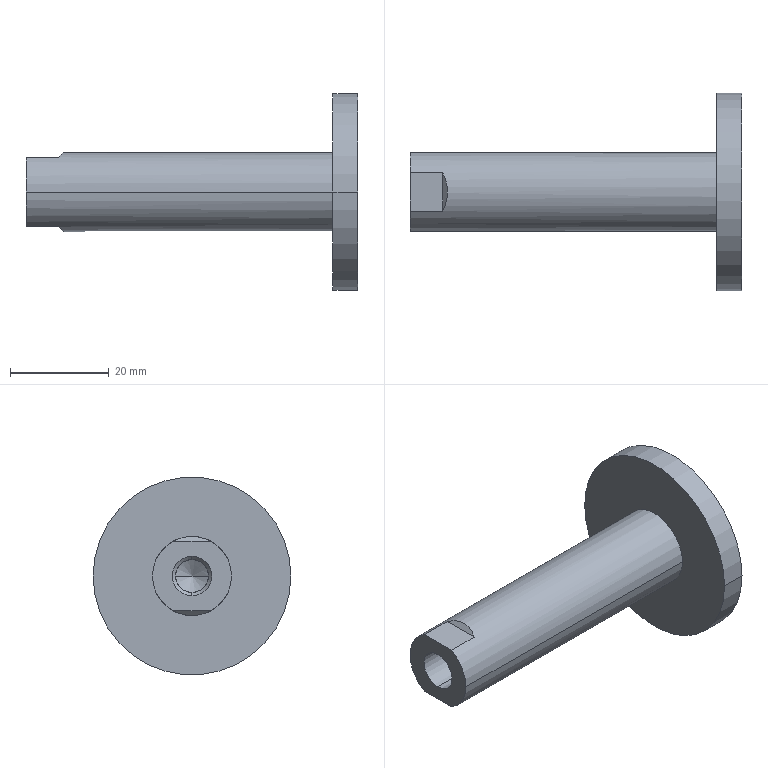Part | STEP file | [25A-CDQ2B40-45C-CYROD] | 1 solid | 19 faces | box 67 x 40 x 40 mm | volume 18078 mm3 | cylinder 8 | plane 7 | cone 4 | commonest cylinder face diameters 6.647 x2 8 x2 16 x2 40 x2
STEP:
#1=CARTESIAN_POINT('',(0.,0.,0.));
#2=DIRECTION('',(0.,0.,1.));
#3=DIRECTION('',(1.,0.,0.));
#4=AXIS2_PLACEMENT_3D('',#1,#2,#3);
#5=CARTESIAN_POINT('',(1.41,0.,-3.323));
#6=VERTEX_POINT('',#5);
#7=CARTESIAN_POINT('',(1.41,3.324,0.));
#8=VERTEX_POINT('',#7);
#9=CARTESIAN_POINT('',(1.41,0.,0.));
#10=DIRECTION('',(1.,0.,0.));
#11=DIRECTION('',(0.,0.,-1.));
#12=AXIS2_PLACEMENT_3D('',#9,#10,#11);
#13=CIRCLE('',#12,3.324);
#14=CARTESIAN_POINT('',(-0.1618,0.,0.));
#15=DIRECTION('',(1.,0.,0.));
#16=DIRECTION('',(0.,1.,0.));
#17=AXIS2_PLACEMENT_3D('',#14,#15,#16);
#18=CYLINDRICAL_SURFACE('',#17,3.324);
#19=CARTESIAN_POINT('',(4.712,1.571));
#20=DIRECTION('',(1.,0.));
#21=VECTOR('',#20,1.);
#22=LINE('',#19,#21);
#23=(GEOMETRIC_REPRESENTATION_CONTEXT(2)PARAMETRIC_REPRESENTATION_CONTEXT()REPRESENTATION_CONTEXT('',''));
#24=DEFINITIONAL_REPRESENTATION('',(#22),#23);
#25=PCURVE('',#18,#24);
#26=CARTESIAN_POINT('',(0.733,0.,0.));
#27=DIRECTION('',(-1.,0.,0.));
#28=DIRECTION('',(0.,0.,-1.));
#29=AXIS2_PLACEMENT_3D('',#26,#27,#28);
#30=CONICAL_SURFACE('',#29,4.,0.7854);
#31=CARTESIAN_POINT('',(6.283,-0.6765));
#32=DIRECTION('',(-1.,0.));
#33=VECTOR('',#32,1.);
#34=LINE('',#31,#33);
#35=(GEOMETRIC_REPRESENTATION_CONTEXT(2)PARAMETRIC_REPRESENTATION_CONTEXT()REPRESENTATION_CONTEXT('',''));
#36=DEFINITIONAL_REPRESENTATION('',(#34),#35);
#37=PCURVE('',#30,#36);
#38=SURFACE_CURVE('',#13,(#25,#37),.PCURVE_S1.);
#39=EDGE_CURVE('',#6,#8,#38,.T.);
#40=ORIENTED_EDGE('',*,*,#39,.T.);
#41=CARTESIAN_POINT('',(6.,3.324,0.));
#42=VERTEX_POINT('',#41);
#43=CARTESIAN_POINT('',(-0.1618,3.324,0.));
#44=DIRECTION('',(1.,0.,0.));
#45=VECTOR('',#44,1.);
#46=LINE('',#43,#45);
#47=CARTESIAN_POINT('',(6.283,0.));
#48=DIRECTION('',(0.,1.));
#49=VECTOR('',#48,1.);
#50=LINE('',#47,#49);
#51=(GEOMETRIC_REPRESENTATION_CONTEXT(2)PARAMETRIC_REPRESENTATION_CONTEXT()REPRESENTATION_CONTEXT('',''));
#52=DEFINITIONAL_REPRESENTATION('',(#50),#51);
#53=PCURVE('',#18,#52);
#54=CARTESIAN_POINT('',(-0.1618,0.,0.));
#55=DIRECTION('',(1.,0.,0.));
#56=DIRECTION('',(0.,1.,0.));
#57=AXIS2_PLACEMENT_3D('',#54,#55,#56);
#58=CYLINDRICAL_SURFACE('',#57,3.324);
#59=CARTESIAN_POINT('',(0.,0.));
#60=DIRECTION('',(0.,1.));
#61=VECTOR('',#60,1.);
#62=LINE('',#59,#61);
#63=(GEOMETRIC_REPRESENTATION_CONTEXT(2)PARAMETRIC_REPRESENTATION_CONTEXT()REPRESENTATION_CONTEXT('',''));
#64=DEFINITIONAL_REPRESENTATION('',(#62),#63);
#65=PCURVE('',#58,#64);
#66=SURFACE_CURVE('',#46,(#53,#65),.PCURVE_S1.);
#67=EDGE_CURVE('',#8,#42,#66,.T.);
#68=ORIENTED_EDGE('',*,*,#67,.T.);
#69=CARTESIAN_POINT('',(6.,-3.324,0.));
#70=VERTEX_POINT('',#69);
#71=CARTESIAN_POINT('',(6.,0.,0.));
#72=DIRECTION('',(-1.,0.,0.));
#73=DIRECTION('',(0.,1.,0.));
#74=AXIS2_PLACEMENT_3D('',#71,#72,#73);
#75=CIRCLE('',#74,3.324);
#76=CARTESIAN_POINT('',(6.283,6.162));
#77=DIRECTION('',(-1.,0.));
#78=VECTOR('',#77,1.);
#79=LINE('',#76,#78);
#80=(GEOMETRIC_REPRESENTATION_CONTEXT(2)PARAMETRIC_REPRESENTATION_CONTEXT()REPRESENTATION_CONTEXT('',''));
#81=DEFINITIONAL_REPRESENTATION('',(#79),#80);
#82=PCURVE('',#18,#81);
#83=CARTESIAN_POINT('',(-992.081,0.,0.));
#84=DIRECTION('',(-1.,0.,0.));
#85=DIRECTION('',(0.,-1.,0.));
#86=AXIS2_PLACEMENT_3D('',#83,#84,#85);
#87=CONICAL_SURFACE('',#86,1732.051,1.047);
#88=CARTESIAN_POINT('',(3.142,-998.081));
#89=DIRECTION('',(1.,0.));
#90=VECTOR('',#89,1.);
#91=LINE('',#88,#90);
#92=(GEOMETRIC_REPRESENTATION_CONTEXT(2)PARAMETRIC_REPRESENTATION_CONTEXT()REPRESENTATION_CONTEXT('',''));
#93=DEFINITIONAL_REPRESENTATION('',(#91),#92);
#94=PCURVE('',#87,#93);
#95=SURFACE_CURVE('',#75,(#82,#94),.PCURVE_S1.);
#96=EDGE_CURVE('',#42,#70,#95,.T.);
#97=ORIENTED_EDGE('',*,*,#96,.T.);
#98=CARTESIAN_POINT('',(1.41,-3.324,0.));
#99=VERTEX_POINT('',#98);
#100=CARTESIAN_POINT('',(-0.1618,-3.324,0.));
#101=DIRECTION('',(1.,0.,0.));
#102=VECTOR('',#101,1.);
#103=LINE('',#100,#102);
#104=CARTESIAN_POINT('',(3.142,0.));
#105=DIRECTION('',(0.,1.));
#106=VECTOR('',#105,1.);
#107=LINE('',#104,#106);
#108=(GEOMETRIC_REPRESENTATION_CONTEXT(2)PARAMETRIC_REPRESENTATION_CONTEXT()REPRESENTATION_CONTEXT('',''));
#109=DEFINITIONAL_REPRESENTATION('',(#107),#108);
#110=PCURVE('',#18,#109);
#111=CARTESIAN_POINT('',(3.142,0.));
#112=DIRECTION('',(0.,1.));
#113=VECTOR('',#112,1.);
#114=LINE('',#111,#113);
#115=(GEOMETRIC_REPRESENTATION_CONTEXT(2)PARAMETRIC_REPRESENTATION_CONTEXT()REPRESENTATION_CONTEXT('',''));
#116=DEFINITIONAL_REPRESENTATION('',(#114),#115);
#117=PCURVE('',#58,#116);
#118=SURFACE_CURVE('',#103,(#110,#117),.PCURVE_S1.);
#119=EDGE_CURVE('',#99,#70,#118,.T.);
#120=ORIENTED_EDGE('',*,*,#119,.F.);
#121=CARTESIAN_POINT('',(1.41,0.,0.));
#122=DIRECTION('',(1.,0.,0.));
#123=DIRECTION('',(0.,0.,-1.));
#124=AXIS2_PLACEMENT_3D('',#121,#122,#123);
#125=CIRCLE('',#124,3.324);
#126=CARTESIAN_POINT('',(-1.571,1.571));
#127=DIRECTION('',(1.,0.));
#128=VECTOR('',#127,1.);
#129=LINE('',#126,#128);
#130=(GEOMETRIC_REPRESENTATION_CONTEXT(2)PARAMETRIC_REPRESENTATION_CONTEXT()REPRESENTATION_CONTEXT('',''));
#131=DEFINITIONAL_REPRESENTATION('',(#129),#130);
#132=PCURVE('',#18,#131);
#133=CARTESIAN_POINT('',(0.733,0.,0.));
#134=DIRECTION('',(-1.,0.,0.));
#135=DIRECTION('',(0.,0.,-1.));
#136=AXIS2_PLACEMENT_3D('',#133,#134,#135);
#137=CONICAL_SURFACE('',#136,4.,0.7854);
#138=CARTESIAN_POINT('',(6.283,-0.6765));
#139=DIRECTION('',(-1.,0.));
#140=VECTOR('',#139,1.);
#141=LINE('',#138,#140);
#142=(GEOMETRIC_REPRESENTATION_CONTEXT(2)PARAMETRIC_REPRESENTATION_CONTEXT()REPRESENTATION_CONTEXT('',''));
#143=DEFINITIONAL_REPRESENTATION('',(#141),#142);
#144=PCURVE('',#137,#143);
#145=SURFACE_CURVE('',#125,(#132,#144),.PCURVE_S1.);
#146=EDGE_CURVE('',#99,#6,#145,.T.);
#147=ORIENTED_EDGE('',*,*,#146,.T.);
#148=EDGE_LOOP('',(#40,#68,#97,#120,#147));
#149=FACE_BOUND('',#148,.F.);
#150=ADVANCED_FACE('',(#149),#18,.F.);
#151=ORIENTED_EDGE('',*,*,#96,.F.);
#152=CARTESIAN_POINT('',(7.919,0.,0.));
#153=VERTEX_POINT('',#152);
#154=CARTESIAN_POINT('',(7.919,0.,0.));
#155=DIRECTION('',(-0.5,0.866,0.));
#156=VECTOR('',#155,1.);
#157=LINE('',#154,#156);
#158=CARTESIAN_POINT('',(3.142,-1000.));
#159=DIRECTION('',(0.,1.));
#160=VECTOR('',#159,1.);
#161=LINE('',#158,#160);
#162=(GEOMETRIC_REPRESENTATION_CONTEXT(2)PARAMETRIC_REPRESENTATION_CONTEXT()REPRESENTATION_CONTEXT('',''));
#163=DEFINITIONAL_REPRESENTATION('',(#161),#162);
#164=PCURVE('',#87,#163);
#165=CARTESIAN_POINT('',(-992.081,0.,0.));
#166=DIRECTION('',(-1.,0.,0.));
#167=DIRECTION('',(0.,-1.,0.));
#168=AXIS2_PLACEMENT_3D('',#165,#166,#167);
#169=CONICAL_SURFACE('',#168,1732.051,1.047);
#170=CARTESIAN_POINT('',(3.142,-1000.));
#171=DIRECTION('',(0.,1.));
#172=VECTOR('',#171,1.);
#173=LINE('',#170,#172);
#174=(GEOMETRIC_REPRESENTATION_CONTEXT(2)PARAMETRIC_REPRESENTATION_CONTEXT()REPRESENTATION_CONTEXT('',''));
#175=DEFINITIONAL_REPRESENTATION('',(#173),#174);
#176=PCURVE('',#169,#175);
#177=SURFACE_CURVE('',#157,(#164,#176),.PCURVE_S1.);
#178=EDGE_CURVE('',#153,#42,#177,.T.);
#179=ORIENTED_EDGE('',*,*,#178,.F.);
#180=CARTESIAN_POINT('',(7.919,0.,0.));
#181=DIRECTION('',(-0.5,-0.866,0.));
#182=VECTOR('',#181,1.);
#183=LINE('',#180,#182);
#184=CARTESIAN_POINT('',(6.283,-1000.));
#185=DIRECTION('',(0.,1.));
#186=VECTOR('',#185,1.);
#187=LINE('',#184,#186);
#188=(GEOMETRIC_REPRESENTATION_CONTEXT(2)PARAMETRIC_REPRESENTATION_CONTEXT()REPRESENTATION_CONTEXT('',''));
#189=DEFINITIONAL_REPRESENTATION('',(#187),#188);
#190=PCURVE('',#87,#189);
#191=CARTESIAN_POINT('',(0.,-1000.));
#192=DIRECTION('',(0.,1.));
#193=VECTOR('',#192,1.);
#194=LINE('',#191,#193);
#195=(GEOMETRIC_REPRESENTATION_CONTEXT(2)PARAMETRIC_REPRESENTATION_CONTEXT()REPRESENTATION_CONTEXT('',''));
#196=DEFINITIONAL_REPRESENTATION('',(#194),#195);
#197=PCURVE('',#169,#196);
#198=SURFACE_CURVE('',#183,(#190,#197),.PCURVE_S1.);
#199=EDGE_CURVE('',#153,#70,#198,.T.);
#200=ORIENTED_EDGE('',*,*,#199,.T.);
#201=EDGE_LOOP('',(#151,#179,#200));
#202=FACE_BOUND('',#201,.F.);
#203=ADVANCED_FACE('',(#202),#87,.F.);
#204=CARTESIAN_POINT('',(-7.,0.,4.));
#205=VERTEX_POINT('',#204);
#206=CARTESIAN_POINT('',(0.733,0.,4.));
#207=VERTEX_POINT('',#206);
#208=CARTESIAN_POINT('',(1.5,0.,4.));
#209=DIRECTION('',(1.,0.,0.));
#210=VECTOR('',#209,1.);
#211=LINE('',#208,#210);
#212=CARTESIAN_POINT('',(1.5,0.,0.));
#213=DIRECTION('',(1.,0.,0.));
#214=DIRECTION('',(0.,0.,1.));
#215=AXIS2_PLACEMENT_3D('',#212,#213,#214);
#216=CYLINDRICAL_SURFACE('',#215,4.);
#217=CARTESIAN_POINT('',(6.283,0.));
#218=DIRECTION('',(0.,1.));
#219=VECTOR('',#218,1.);
#220=LINE('',#217,#219);
#221=(GEOMETRIC_REPRESENTATION_CONTEXT(2)PARAMETRIC_REPRESENTATION_CONTEXT()REPRESENTATION_CONTEXT('',''));
#222=DEFINITIONAL_REPRESENTATION('',(#220),#221);
#223=PCURVE('',#216,#222);
#224=CARTESIAN_POINT('',(1.5,0.,0.));
#225=DIRECTION('',(1.,0.,0.));
#226=DIRECTION('',(0.,0.,1.));
#227=AXIS2_PLACEMENT_3D('',#224,#225,#226);
#228=CYLINDRICAL_SURFACE('',#227,4.);
#229=CARTESIAN_POINT('',(0.,0.));
#230=DIRECTION('',(0.,1.));
#231=VECTOR('',#230,1.);
#232=LINE('',#229,#231);
#233=(GEOMETRIC_REPRESENTATION_CONTEXT(2)PARAMETRIC_REPRESENTATION_CONTEXT()REPRESENTATION_CONTEXT('',''));
#234=DEFINITIONAL_REPRESENTATION('',(#232),#233);
#235=PCURVE('',#228,#234);
#236=SURFACE_CURVE('',#211,(#223,#235),.PCURVE_S1.);
#237=EDGE_CURVE('',#205,#207,#236,.T.);
#238=ORIENTED_EDGE('',*,*,#237,.T.);
#239=CARTESIAN_POINT('',(0.733,0.,-4.));
#240=VERTEX_POINT('',#239);
#241=CARTESIAN_POINT('',(0.733,0.,0.));
#242=DIRECTION('',(1.,0.,0.));
#243=DIRECTION('',(0.,0.,1.));
#244=AXIS2_PLACEMENT_3D('',#241,#242,#243);
#245=CIRCLE('',#244,4.);
#246=CARTESIAN_POINT('',(0.,-0.767));
#247=DIRECTION('',(1.,0.));
#248=VECTOR('',#247,1.);
#249=LINE('',#246,#248);
#250=(GEOMETRIC_REPRESENTATION_CONTEXT(2)PARAMETRIC_REPRESENTATION_CONTEXT()REPRESENTATION_CONTEXT('',''));
#251=DEFINITIONAL_REPRESENTATION('',(#249),#250);
#252=PCURVE('',#216,#251);
#253=CARTESIAN_POINT('',(9.425,0.));
#254=DIRECTION('',(-1.,0.));
#255=VECTOR('',#254,1.);
#256=LINE('',#253,#255);
#257=(GEOMETRIC_REPRESENTATION_CONTEXT(2)PARAMETRIC_REPRESENTATION_CONTEXT()REPRESENTATION_CONTEXT('',''));
#258=DEFINITIONAL_REPRESENTATION('',(#256),#257);
#259=PCURVE('',#30,#258);
#260=SURFACE_CURVE('',#245,(#252,#259),.PCURVE_S1.);
#261=EDGE_CURVE('',#240,#207,#260,.T.);
#262=ORIENTED_EDGE('',*,*,#261,.F.);
#263=CARTESIAN_POINT('',(-7.,0.,-4.));
#264=VERTEX_POINT('',#263);
#265=CARTESIAN_POINT('',(1.5,0.,-4.));
#266=DIRECTION('',(1.,0.,0.));
#267=VECTOR('',#266,1.);
#268=LINE('',#265,#267);
#269=CARTESIAN_POINT('',(3.142,0.));
#270=DIRECTION('',(0.,1.));
#271=VECTOR('',#270,1.);
#272=LINE('',#269,#271);
#273=(GEOMETRIC_REPRESENTATION_CONTEXT(2)PARAMETRIC_REPRESENTATION_CONTEXT()REPRESENTATION_CONTEXT('',''));
#274=DEFINITIONAL_REPRESENTATION('',(#272),#273);
#275=PCURVE('',#216,#274);
#276=CARTESIAN_POINT('',(3.142,0.));
#277=DIRECTION('',(0.,1.));
#278=VECTOR('',#277,1.);
#279=LINE('',#276,#278);
#280=(GEOMETRIC_REPRESENTATION_CONTEXT(2)PARAMETRIC_REPRESENTATION_CONTEXT()REPRESENTATION_CONTEXT('',''));
#281=DEFINITIONAL_REPRESENTATION('',(#279),#280);
#282=PCURVE('',#228,#281);
#283=SURFACE_CURVE('',#268,(#275,#282),.PCURVE_S1.);
#284=EDGE_CURVE('',#264,#240,#283,.T.);
#285=ORIENTED_EDGE('',*,*,#284,.F.);
#286=CARTESIAN_POINT('',(-7.,0.,0.));
#287=DIRECTION('',(1.,0.,0.));
#288=DIRECTION('',(0.,1.,0.));
#289=AXIS2_PLACEMENT_3D('',#286,#287,#288);
#290=CIRCLE('',#289,4.);
#291=CARTESIAN_POINT('',(-1.571,-8.5));
#292=DIRECTION('',(1.,0.));
#293=VECTOR('',#292,1.);
#294=LINE('',#291,#293);
#295=(GEOMETRIC_REPRESENTATION_CONTEXT(2)PARAMETRIC_REPRESENTATION_CONTEXT()REPRESENTATION_CONTEXT('',''));
#296=DEFINITIONAL_REPRESENTATION('',(#294),#295);
#297=PCURVE('',#216,#296);
#298=CARTESIAN_POINT('',(-7.,-15.945,-15.945));
#299=DIRECTION('',(1.,0.,0.));
#300=DIRECTION('',(0.,1.,0.));
#301=AXIS2_PLACEMENT_3D('',#298,#299,#300);
#302=PLANE('',#301);
#303=CARTESIAN_POINT('',(15.945,15.945));
#304=DIRECTION('',(1.,0.));
#305=AXIS2_PLACEMENT_2D('',#303,#304);
#306=CIRCLE('',#305,4.);
#307=(GEOMETRIC_REPRESENTATION_CONTEXT(2)PARAMETRIC_REPRESENTATION_CONTEXT()REPRESENTATION_CONTEXT('',''));
#308=DEFINITIONAL_REPRESENTATION('',(#306),#307);
#309=PCURVE('',#302,#308);
#310=SURFACE_CURVE('',#290,(#297,#309),.PCURVE_S1.);
#311=EDGE_CURVE('',#264,#205,#310,.T.);
#312=ORIENTED_EDGE('',*,*,#311,.T.);
#313=EDGE_LOOP('',(#238,#262,#285,#312));
#314=FACE_BOUND('',#313,.F.);
#315=ADVANCED_FACE('',(#314),#216,.F.);
#316=CARTESIAN_POINT('',(0.733,0.,-4.));
#317=DIRECTION('',(-0.7071,0.,-0.7071));
#318=VECTOR('',#317,1.);
#319=LINE('',#316,#318);
#320=CARTESIAN_POINT('',(6.283,0.));
#321=DIRECTION('',(0.,1.));
#322=VECTOR('',#321,1.);
#323=LINE('',#320,#322);
#324=(GEOMETRIC_REPRESENTATION_CONTEXT(2)PARAMETRIC_REPRESENTATION_CONTEXT()REPRESENTATION_CONTEXT('',''));
#325=DEFINITIONAL_REPRESENTATION('',(#323),#324);
#326=PCURVE('',#30,#325);
#327=CARTESIAN_POINT('',(0.,0.));
#328=DIRECTION('',(0.,1.));
#329=VECTOR('',#328,1.);
#330=LINE('',#327,#329);
#331=(GEOMETRIC_REPRESENTATION_CONTEXT(2)PARAMETRIC_REPRESENTATION_CONTEXT()REPRESENTATION_CONTEXT('',''));
#332=DEFINITIONAL_REPRESENTATION('',(#330),#331);
#333=PCURVE('',#137,#332);
#334=SURFACE_CURVE('',#319,(#326,#333),.PCURVE_S1.);
#335=EDGE_CURVE('',#6,#240,#334,.T.);
#336=ORIENTED_EDGE('',*,*,#335,.T.);
#337=ORIENTED_EDGE('',*,*,#261,.T.);
#338=CARTESIAN_POINT('',(1.41,0.,3.324));
#339=VERTEX_POINT('',#338);
#340=CARTESIAN_POINT('',(0.733,0.,4.));
#341=DIRECTION('',(-0.7071,0.,0.7071));
#342=VECTOR('',#341,1.);
#343=LINE('',#340,#342);
#344=CARTESIAN_POINT('',(3.142,0.));
#345=DIRECTION('',(0.,1.));
#346=VECTOR('',#345,1.);
#347=LINE('',#344,#346);
#348=(GEOMETRIC_REPRESENTATION_CONTEXT(2)PARAMETRIC_REPRESENTATION_CONTEXT()REPRESENTATION_CONTEXT('',''));
#349=DEFINITIONAL_REPRESENTATION('',(#347),#348);
#350=PCURVE('',#30,#349);
#351=CARTESIAN_POINT('',(3.142,0.));
#352=DIRECTION('',(0.,1.));
#353=VECTOR('',#352,1.);
#354=LINE('',#351,#353);
#355=(GEOMETRIC_REPRESENTATION_CONTEXT(2)PARAMETRIC_REPRESENTATION_CONTEXT()REPRESENTATION_CONTEXT('',''));
#356=DEFINITIONAL_REPRESENTATION('',(#354),#355);
#357=PCURVE('',#137,#356);
#358=SURFACE_CURVE('',#343,(#350,#357),.PCURVE_S1.);
#359=EDGE_CURVE('',#339,#207,#358,.T.);
#360=ORIENTED_EDGE('',*,*,#359,.F.);
#361=CARTESIAN_POINT('',(1.41,0.,0.));
#362=DIRECTION('',(1.,0.,0.));
#363=DIRECTION('',(0.,0.,-1.));
#364=AXIS2_PLACEMENT_3D('',#361,#362,#363);
#365=CIRCLE('',#364,3.324);
#366=CARTESIAN_POINT('',(6.283,-0.6765));
#367=DIRECTION('',(-1.,0.));
#368=VECTOR('',#367,1.);
#369=LINE('',#366,#368);
#370=(GEOMETRIC_REPRESENTATION_CONTEXT(2)PARAMETRIC_REPRESENTATION_CONTEXT()REPRESENTATION_CONTEXT('',''));
#371=DEFINITIONAL_REPRESENTATION('',(#369),#370);
#372=PCURVE('',#30,#371);
#373=CARTESIAN_POINT('',(-1.571,1.571));
#374=DIRECTION('',(1.,0.));
#375=VECTOR('',#374,1.);
#376=LINE('',#373,#375);
#377=(GEOMETRIC_REPRESENTATION_CONTEXT(2)PARAMETRIC_REPRESENTATION_CONTEXT()REPRESENTATION_CONTEXT('',''));
#378=DEFINITIONAL_REPRESENTATION('',(#376),#377);
#379=PCURVE('',#58,#378);
#380=SURFACE_CURVE('',#365,(#372,#379),.PCURVE_S1.);
#381=EDGE_CURVE('',#8,#339,#380,.T.);
#382=ORIENTED_EDGE('',*,*,#381,.F.);
#383=ORIENTED_EDGE('',*,*,#39,.F.);
#384=EDGE_LOOP('',(#336,#337,#360,#382,#383));
#385=FACE_BOUND('',#384,.F.);
#386=ADVANCED_FACE('',(#385),#30,.F.);
#387=CARTESIAN_POINT('',(55.,-20.,0.));
#388=VERTEX_POINT('',#387);
#389=CARTESIAN_POINT('',(55.,20.,0.));
#390=VERTEX_POINT('',#389);
#391=CARTESIAN_POINT('',(55.,0.,0.));
#392=DIRECTION('',(-1.,0.,0.));
#393=DIRECTION('',(0.,1.,0.));
#394=AXIS2_PLACEMENT_3D('',#391,#392,#393);
#395=CIRCLE('',#394,20.);
#396=CARTESIAN_POINT('',(57.5,0.,0.));
#397=DIRECTION('',(1.,0.,0.));
#398=DIRECTION('',(0.,1.,0.));
#399=AXIS2_PLACEMENT_3D('',#396,#397,#398);
#400=CYLINDRICAL_SURFACE('',#399,20.);
#401=CARTESIAN_POINT('',(6.283,-2.5));
#402=DIRECTION('',(-1.,0.));
#403=VECTOR('',#402,1.);
#404=LINE('',#401,#403);
#405=(GEOMETRIC_REPRESENTATION_CONTEXT(2)PARAMETRIC_REPRESENTATION_CONTEXT()REPRESENTATION_CONTEXT('',''));
#406=DEFINITIONAL_REPRESENTATION('',(#404),#405);
#407=PCURVE('',#400,#406);
#408=CARTESIAN_POINT('',(55.,-42.426,-42.426));
#409=DIRECTION('',(1.,0.,0.));
#410=DIRECTION('',(0.,1.,0.));
#411=AXIS2_PLACEMENT_3D('',#408,#409,#410);
#412=PLANE('',#411);
#413=CARTESIAN_POINT('',(62.426,42.426));
#414=CARTESIAN_POINT('',(62.426,7.785));
#415=CARTESIAN_POINT('',(32.426,25.106));
#416=CARTESIAN_POINT('',(2.426,42.426));
#417=CARTESIAN_POINT('',(32.426,59.747));
#418=CARTESIAN_POINT('',(62.426,77.067));
#419=CARTESIAN_POINT('',(62.426,42.426));
#420=(BOUNDED_CURVE()B_SPLINE_CURVE(2,(#413,#414,#415,#416,#417,#418,#419),.UNSPECIFIED.,.T.,.F.)B_SPLINE_CURVE_WITH_KNOTS((1,2,2,2,2,1),(-2.094,0.,2.094,4.189,6.283,8.378),.UNSPECIFIED.)CURVE()GEOMETRIC_REPRESENTATION_ITEM()RATIONAL_B_SPLINE_CURVE((1.,0.5,1.,0.5,1.,0.5,1.))REPRESENTATION_ITEM(''));
#421=(GEOMETRIC_REPRESENTATION_CONTEXT(2)PARAMETRIC_REPRESENTATION_CONTEXT()REPRESENTATION_CONTEXT('',''));
#422=DEFINITIONAL_REPRESENTATION('',(#420),#421);
#423=PCURVE('',#412,#422);
#424=SURFACE_CURVE('',#395,(#407,#423),.PCURVE_S1.);
#425=EDGE_CURVE('',#388,#390,#424,.T.);
#426=ORIENTED_EDGE('',*,*,#425,.F.);
#427=CARTESIAN_POINT('',(60.,-20.,0.));
#428=VERTEX_POINT('',#427);
#429=CARTESIAN_POINT('',(57.5,-20.,0.));
#430=DIRECTION('',(1.,0.,0.));
#431=VECTOR('',#430,1.);
#432=LINE('',#429,#431);
#433=CARTESIAN_POINT('',(3.142,0.));
#434=DIRECTION('',(0.,1.));
#435=VECTOR('',#434,1.);
#436=LINE('',#433,#435);
#437=(GEOMETRIC_REPRESENTATION_CONTEXT(2)PARAMETRIC_REPRESENTATION_CONTEXT()REPRESENTATION_CONTEXT('',''));
#438=DEFINITIONAL_REPRESENTATION('',(#436),#437);
#439=PCURVE('',#400,#438);
#440=CARTESIAN_POINT('',(57.5,0.,0.));
#441=DIRECTION('',(1.,0.,0.));
#442=DIRECTION('',(0.,1.,0.));
#443=AXIS2_PLACEMENT_3D('',#440,#441,#442);
#444=CYLINDRICAL_SURFACE('',#443,20.);
#445=CARTESIAN_POINT('',(3.142,0.));
#446=DIRECTION('',(0.,1.));
#447=VECTOR('',#446,1.);
#448=LINE('',#445,#447);
#449=(GEOMETRIC_REPRESENTATION_CONTEXT(2)PARAMETRIC_REPRESENTATION_CONTEXT()REPRESENTATION_CONTEXT('',''));
#450=DEFINITIONAL_REPRESENTATION('',(#448),#449);
#451=PCURVE('',#444,#450);
#452=SURFACE_CURVE('',#432,(#439,#451),.PCURVE_S1.);
#453=EDGE_CURVE('',#388,#428,#452,.T.);
#454=ORIENTED_EDGE('',*,*,#453,.T.);
#455=CARTESIAN_POINT('',(60.,20.,0.));
#456=VERTEX_POINT('',#455);
#457=CARTESIAN_POINT('',(60.,0.,0.));
#458=DIRECTION('',(1.,0.,0.));
#459=DIRECTION('',(0.,-1.,0.));
#460=AXIS2_PLACEMENT_3D('',#457,#458,#459);
#461=CIRCLE('',#460,20.);
#462=CARTESIAN_POINT('',(-3.142,2.5));
#463=DIRECTION('',(1.,0.));
#464=VECTOR('',#463,1.);
#465=LINE('',#462,#464);
#466=(GEOMETRIC_REPRESENTATION_CONTEXT(2)PARAMETRIC_REPRESENTATION_CONTEXT()REPRESENTATION_CONTEXT('',''));
#467=DEFINITIONAL_REPRESENTATION('',(#465),#466);
#468=PCURVE('',#400,#467);
#469=CARTESIAN_POINT('',(60.,42.426,-42.426));
#470=DIRECTION('',(-1.,0.,0.));
#471=DIRECTION('',(0.,-1.,0.));
#472=AXIS2_PLACEMENT_3D('',#469,#470,#471);
#473=PLANE('',#472);
#474=CARTESIAN_POINT('',(62.426,42.426));
#475=CARTESIAN_POINT('',(62.426,7.785));
#476=CARTESIAN_POINT('',(32.426,25.106));
#477=CARTESIAN_POINT('',(2.426,42.426));
#478=CARTESIAN_POINT('',(32.426,59.747));
#479=CARTESIAN_POINT('',(62.426,77.067));
#480=CARTESIAN_POINT('',(62.426,42.426));
#481=(BOUNDED_CURVE()B_SPLINE_CURVE(2,(#474,#475,#476,#477,#478,#479,#480),.UNSPECIFIED.,.T.,.F.)B_SPLINE_CURVE_WITH_KNOTS((1,2,2,2,2,1),(-2.094,0.,2.094,4.189,6.283,8.378),.UNSPECIFIED.)CURVE()GEOMETRIC_REPRESENTATION_ITEM()RATIONAL_B_SPLINE_CURVE((1.,0.5,1.,0.5,1.,0.5,1.))REPRESENTATION_ITEM(''));
#482=(GEOMETRIC_REPRESENTATION_CONTEXT(2)PARAMETRIC_REPRESENTATION_CONTEXT()REPRESENTATION_CONTEXT('',''));
#483=DEFINITIONAL_REPRESENTATION('',(#481),#482);
#484=PCURVE('',#473,#483);
#485=SURFACE_CURVE('',#461,(#468,#484),.PCURVE_S1.);
#486=EDGE_CURVE('',#456,#428,#485,.T.);
#487=ORIENTED_EDGE('',*,*,#486,.F.);
#488=CARTESIAN_POINT('',(57.5,20.,0.));
#489=DIRECTION('',(1.,0.,0.));
#490=VECTOR('',#489,1.);
#491=LINE('',#488,#490);
#492=CARTESIAN_POINT('',(0.,0.));
#493=DIRECTION('',(0.,1.));
#494=VECTOR('',#493,1.);
#495=LINE('',#492,#494);
#496=(GEOMETRIC_REPRESENTATION_CONTEXT(2)PARAMETRIC_REPRESENTATION_CONTEXT()REPRESENTATION_CONTEXT('',''));
#497=DEFINITIONAL_REPRESENTATION('',(#495),#496);
#498=PCURVE('',#400,#497);
#499=CARTESIAN_POINT('',(6.283,0.));
#500=DIRECTION('',(0.,1.));
#501=VECTOR('',#500,1.);
#502=LINE('',#499,#501);
#503=(GEOMETRIC_REPRESENTATION_CONTEXT(2)PARAMETRIC_REPRESENTATION_CONTEXT()REPRESENTATION_CONTEXT('',''));
#504=DEFINITIONAL_REPRESENTATION('',(#502),#503);
#505=PCURVE('',#444,#504);
#506=SURFACE_CURVE('',#491,(#498,#505),.PCURVE_S1.);
#507=EDGE_CURVE('',#390,#456,#506,.T.);
#508=ORIENTED_EDGE('',*,*,#507,.F.);
#509=EDGE_LOOP('',(#426,#454,#487,#508));
#510=FACE_BOUND('',#509,.T.);
#511=ADVANCED_FACE('',(#510),#400,.T.);
#512=CARTESIAN_POINT('',(-7.,-8.,0.));
#513=VERTEX_POINT('',#512);
#514=CARTESIAN_POINT('',(-7.,-3.873,7.));
#515=VERTEX_POINT('',#514);
#516=CARTESIAN_POINT('',(-7.,0.,0.));
#517=DIRECTION('',(-1.,0.,0.));
#518=DIRECTION('',(0.,-1.,0.));
#519=AXIS2_PLACEMENT_3D('',#516,#517,#518);
#520=CIRCLE('',#519,8.);
#521=CARTESIAN_POINT('',(24.,0.,0.));
#522=DIRECTION('',(1.,0.,0.));
#523=DIRECTION('',(0.,1.,0.));
#524=AXIS2_PLACEMENT_3D('',#521,#522,#523);
#525=CYLINDRICAL_SURFACE('',#524,8.);
#526=CARTESIAN_POINT('',(3.142,-31.));
#527=DIRECTION('',(-1.,0.));
#528=VECTOR('',#527,1.);
#529=LINE('',#526,#528);
#530=(GEOMETRIC_REPRESENTATION_CONTEXT(2)PARAMETRIC_REPRESENTATION_CONTEXT()REPRESENTATION_CONTEXT('',''));
#531=DEFINITIONAL_REPRESENTATION('',(#529),#530);
#532=PCURVE('',#525,#531);
#533=CARTESIAN_POINT('',(7.945,15.945));
#534=CARTESIAN_POINT('',(7.945,29.802));
#535=CARTESIAN_POINT('',(19.945,22.873));
#536=CARTESIAN_POINT('',(31.945,15.945));
#537=CARTESIAN_POINT('',(19.945,9.017));
#538=CARTESIAN_POINT('',(7.945,2.089));
#539=CARTESIAN_POINT('',(7.945,15.945));
#540=(BOUNDED_CURVE()B_SPLINE_CURVE(2,(#533,#534,#535,#536,#537,#538,#539),.UNSPECIFIED.,.T.,.F.)B_SPLINE_CURVE_WITH_KNOTS((1,2,2,2,2,1),(-2.094,0.,2.094,4.189,6.283,8.378),.UNSPECIFIED.)CURVE()GEOMETRIC_REPRESENTATION_ITEM()RATIONAL_B_SPLINE_CURVE((1.,0.5,1.,0.5,1.,0.5,1.))REPRESENTATION_ITEM(''));
#541=(GEOMETRIC_REPRESENTATION_CONTEXT(2)PARAMETRIC_REPRESENTATION_CONTEXT()REPRESENTATION_CONTEXT('',''));
#542=DEFINITIONAL_REPRESENTATION('',(#540),#541);
#543=PCURVE('',#302,#542);
#544=SURFACE_CURVE('',#520,(#532,#543),.PCURVE_S1.);
#545=EDGE_CURVE('',#513,#515,#544,.T.);
#546=ORIENTED_EDGE('',*,*,#545,.F.);
#547=CARTESIAN_POINT('',(55.,-8.,0.));
#548=VERTEX_POINT('',#547);
#549=CARTESIAN_POINT('',(24.,-8.,0.));
#550=DIRECTION('',(1.,0.,0.));
#551=VECTOR('',#550,1.);
#552=LINE('',#549,#551);
#553=CARTESIAN_POINT('',(3.142,0.));
#554=DIRECTION('',(0.,1.));
#555=VECTOR('',#554,1.);
#556=LINE('',#553,#555);
#557=(GEOMETRIC_REPRESENTATION_CONTEXT(2)PARAMETRIC_REPRESENTATION_CONTEXT()REPRESENTATION_CONTEXT('',''));
#558=DEFINITIONAL_REPRESENTATION('',(#556),#557);
#559=PCURVE('',#525,#558);
#560=CARTESIAN_POINT('',(24.,0.,0.));
#561=DIRECTION('',(1.,0.,0.));
#562=DIRECTION('',(0.,1.,0.));
#563=AXIS2_PLACEMENT_3D('',#560,#561,#562);
#564=CYLINDRICAL_SURFACE('',#563,8.);
#565=CARTESIAN_POINT('',(3.142,0.));
#566=DIRECTION('',(0.,1.));
#567=VECTOR('',#566,1.);
#568=LINE('',#565,#567);
#569=(GEOMETRIC_REPRESENTATION_CONTEXT(2)PARAMETRIC_REPRESENTATION_CONTEXT()REPRESENTATION_CONTEXT('',''));
#570=DEFINITIONAL_REPRESENTATION('',(#568),#569);
#571=PCURVE('',#564,#570);
#572=SURFACE_CURVE('',#552,(#559,#571),.PCURVE_S1.);
#573=EDGE_CURVE('',#513,#548,#572,.T.);
#574=ORIENTED_EDGE('',*,*,#573,.T.);
#575=CARTESIAN_POINT('',(55.,8.,0.));
#576=VERTEX_POINT('',#575);
#577=CARTESIAN_POINT('',(55.,0.,0.));
#578=DIRECTION('',(1.,0.,0.));
#579=DIRECTION('',(0.,-1.,0.));
#580=AXIS2_PLACEMENT_3D('',#577,#578,#579);
#581=CIRCLE('',#580,8.);
#582=CARTESIAN_POINT('',(-3.142,31.));
#583=DIRECTION('',(1.,0.));
#584=VECTOR('',#583,1.);
#585=LINE('',#582,#584);
#586=(GEOMETRIC_REPRESENTATION_CONTEXT(2)PARAMETRIC_REPRESENTATION_CONTEXT()REPRESENTATION_CONTEXT('',''));
#587=DEFINITIONAL_REPRESENTATION('',(#585),#586);
#588=PCURVE('',#525,#587);
#589=CARTESIAN_POINT('',(42.426,42.426));
#590=DIRECTION('',(-1.,0.));
#591=AXIS2_PLACEMENT_2D('',#589,#590);
#592=CIRCLE('',#591,8.);
#593=(GEOMETRIC_REPRESENTATION_CONTEXT(2)PARAMETRIC_REPRESENTATION_CONTEXT()REPRESENTATION_CONTEXT('',''));
#594=DEFINITIONAL_REPRESENTATION('',(#592),#593);
#595=PCURVE('',#412,#594);
#596=SURFACE_CURVE('',#581,(#588,#595),.PCURVE_S1.);
#597=EDGE_CURVE('',#576,#548,#596,.T.);
#598=ORIENTED_EDGE('',*,*,#597,.F.);
#599=CARTESIAN_POINT('',(-7.,8.,0.));
#600=VERTEX_POINT('',#599);
#601=CARTESIAN_POINT('',(24.,8.,0.));
#602=DIRECTION('',(1.,0.,0.));
#603=VECTOR('',#602,1.);
#604=LINE('',#601,#603);
#605=CARTESIAN_POINT('',(0.,0.));
#606=DIRECTION('',(0.,1.));
#607=VECTOR('',#606,1.);
#608=LINE('',#605,#607);
#609=(GEOMETRIC_REPRESENTATION_CONTEXT(2)PARAMETRIC_REPRESENTATION_CONTEXT()REPRESENTATION_CONTEXT('',''));
#610=DEFINITIONAL_REPRESENTATION('',(#608),#609);
#611=PCURVE('',#525,#610);
#612=CARTESIAN_POINT('',(6.283,0.));
#613=DIRECTION('',(0.,1.));
#614=VECTOR('',#613,1.);
#615=LINE('',#612,#614);
#616=(GEOMETRIC_REPRESENTATION_CONTEXT(2)PARAMETRIC_REPRESENTATION_CONTEXT()REPRESENTATION_CONTEXT('',''));
#617=DEFINITIONAL_REPRESENTATION('',(#615),#616);
#618=PCURVE('',#564,#617);
#619=SURFACE_CURVE('',#604,(#611,#618),.PCURVE_S1.);
#620=EDGE_CURVE('',#600,#576,#619,.T.);
#621=ORIENTED_EDGE('',*,*,#620,.F.);
#622=CARTESIAN_POINT('',(-7.,3.873,7.));
#623=VERTEX_POINT('',#622);
#624=CARTESIAN_POINT('',(-7.,0.,0.));
#625=DIRECTION('',(-1.,0.,0.));
#626=DIRECTION('',(0.,1.,0.));
#627=AXIS2_PLACEMENT_3D('',#624,#625,#626);
#628=CIRCLE('',#627,8.);
#629=CARTESIAN_POINT('',(6.283,-31.));
#630=DIRECTION('',(-1.,0.));
#631=VECTOR('',#630,1.);
#632=LINE('',#629,#631);
#633=(GEOMETRIC_REPRESENTATION_CONTEXT(2)PARAMETRIC_REPRESENTATION_CONTEXT()REPRESENTATION_CONTEXT('',''));
#634=DEFINITIONAL_REPRESENTATION('',(#632),#633);
#635=PCURVE('',#525,#634);
#636=CARTESIAN_POINT('',(23.945,15.945));
#637=CARTESIAN_POINT('',(23.945,2.089));
#638=CARTESIAN_POINT('',(11.945,9.017));
#639=CARTESIAN_POINT('',(-0.05478,15.945));
#640=CARTESIAN_POINT('',(11.945,22.873));
#641=CARTESIAN_POINT('',(23.945,29.802));
#642=CARTESIAN_POINT('',(23.945,15.945));
#643=(BOUNDED_CURVE()B_SPLINE_CURVE(2,(#636,#637,#638,#639,#640,#641,#642),.UNSPECIFIED.,.T.,.F.)B_SPLINE_CURVE_WITH_KNOTS((1,2,2,2,2,1),(-2.094,0.,2.094,4.189,6.283,8.378),.UNSPECIFIED.)CURVE()GEOMETRIC_REPRESENTATION_ITEM()RATIONAL_B_SPLINE_CURVE((1.,0.5,1.,0.5,1.,0.5,1.))REPRESENTATION_ITEM(''));
#644=(GEOMETRIC_REPRESENTATION_CONTEXT(2)PARAMETRIC_REPRESENTATION_CONTEXT()REPRESENTATION_CONTEXT('',''));
#645=DEFINITIONAL_REPRESENTATION('',(#643),#644);
#646=PCURVE('',#302,#645);
#647=SURFACE_CURVE('',#628,(#635,#646),.PCURVE_S1.);
#648=EDGE_CURVE('',#623,#600,#647,.T.);
#649=ORIENTED_EDGE('',*,*,#648,.F.);
#650=CARTESIAN_POINT('',(-0.5,3.873,7.));
#651=VERTEX_POINT('',#650);
#652=CARTESIAN_POINT('',(-7.,3.873,7.));
#653=DIRECTION('',(1.,0.,0.));
#654=VECTOR('',#653,1.);
#655=LINE('',#652,#654);
#656=CARTESIAN_POINT('',(1.065,-31.));
#657=DIRECTION('',(0.,1.));
#658=VECTOR('',#657,1.);
#659=LINE('',#656,#658);
#660=(GEOMETRIC_REPRESENTATION_CONTEXT(2)PARAMETRIC_REPRESENTATION_CONTEXT()REPRESENTATION_CONTEXT('',''));
#661=DEFINITIONAL_REPRESENTATION('',(#659),#660);
#662=PCURVE('',#525,#661);
#663=CARTESIAN_POINT('',(-11.334,-7.584,7.));
#664=DIRECTION('',(0.,0.,1.));
#665=DIRECTION('',(1.,0.,0.));
#666=AXIS2_PLACEMENT_3D('',#663,#664,#665);
#667=PLANE('',#666);
#668=CARTESIAN_POINT('',(4.334,11.457));
#669=DIRECTION('',(1.,0.));
#670=VECTOR('',#669,1.);
#671=LINE('',#668,#670);
#672=(GEOMETRIC_REPRESENTATION_CONTEXT(2)PARAMETRIC_REPRESENTATION_CONTEXT()REPRESENTATION_CONTEXT('',''));
#673=DEFINITIONAL_REPRESENTATION('',(#671),#672);
#674=PCURVE('',#667,#673);
#675=SURFACE_CURVE('',#655,(#662,#674),.PCURVE_S1.);
#676=EDGE_CURVE('',#623,#651,#675,.T.);
#677=ORIENTED_EDGE('',*,*,#676,.T.);
#678=CARTESIAN_POINT('',(-0.5,-3.873,7.));
#679=VERTEX_POINT('',#678);
#680=CARTESIAN_POINT('',(-0.5,3.873,7.));
#681=CARTESIAN_POINT('',(-0.1909,3.328,7.302));
#682=CARTESIAN_POINT('',(0.05915,2.712,7.557));
#683=CARTESIAN_POINT('',(0.4046,1.398,7.906));
#684=CARTESIAN_POINT('',(0.5,0.6991,8.));
#685=CARTESIAN_POINT('',(0.5,-0.6991,8.));
#686=CARTESIAN_POINT('',(0.4046,-1.398,7.906));
#687=CARTESIAN_POINT('',(0.05915,-2.712,7.557));
#688=CARTESIAN_POINT('',(-0.1909,-3.328,7.302));
#689=CARTESIAN_POINT('',(-0.5,-3.873,7.));
#690=B_SPLINE_CURVE_WITH_KNOTS('',3,(#680,#681,#682,#683,#684,#685,#686,#687,#688,#689),.UNSPECIFIED.,.F.,.F.,(4,2,2,2,4),(0.,0.25,0.5,0.75,1.),.UNSPECIFIED.);
#691=CARTESIAN_POINT('',(1.065,-24.5));
#692=CARTESIAN_POINT('',(1.08,-24.444));
#693=CARTESIAN_POINT('',(1.108,-24.335));
#694=CARTESIAN_POINT('',(1.152,-24.185));
#695=CARTESIAN_POINT('',(1.197,-24.048));
#696=CARTESIAN_POINT('',(1.242,-23.924));
#697=CARTESIAN_POINT('',(1.288,-23.815));
#698=CARTESIAN_POINT('',(1.334,-23.72));
#699=CARTESIAN_POINT('',(1.381,-23.642));
#700=CARTESIAN_POINT('',(1.428,-23.579));
#701=CARTESIAN_POINT('',(1.476,-23.534));
#702=CARTESIAN_POINT('',(1.523,-23.506));
#703=CARTESIAN_POINT('',(1.571,-23.497));
#704=CARTESIAN_POINT('',(1.618,-23.506));
#705=CARTESIAN_POINT('',(1.666,-23.534));
#706=CARTESIAN_POINT('',(1.713,-23.579));
#707=CARTESIAN_POINT('',(1.761,-23.642));
#708=CARTESIAN_POINT('',(1.807,-23.72));
#709=CARTESIAN_POINT('',(1.854,-23.815));
#710=CARTESIAN_POINT('',(1.9,-23.924));
#711=CARTESIAN_POINT('',(1.945,-24.048));
#712=CARTESIAN_POINT('',(1.99,-24.185));
#713=CARTESIAN_POINT('',(2.033,-24.335));
#714=CARTESIAN_POINT('',(2.062,-24.444));
#715=CARTESIAN_POINT('',(2.076,-24.5));
#716=B_SPLINE_CURVE_WITH_KNOTS('',3,(#691,#692,#693,#694,#695,#696,#697,#698,#699,#700,#701,#702,#703,#704,#705,#706,#707,#708,#709,#710,#711,#712,#713,#714,#715),.UNSPECIFIED.,.F.,.F.,(4,1,1,1,1,1,1,1,1,1,1,1,1,1,1,1,1,1,1,1,1,1,4),(0.,0.04545,0.09091,0.1364,0.1818,0.2273,0.2727,0.3182,0.3636,0.4091,0.4545,0.5,0.5455,0.5909,0.6364,0.6818,0.7273,0.7727,0.8182,0.8636,0.9091,0.9545,1.),.QUASI_UNIFORM_KNOTS.);
#717=(GEOMETRIC_REPRESENTATION_CONTEXT(2)PARAMETRIC_REPRESENTATION_CONTEXT()REPRESENTATION_CONTEXT('',''));
#718=DEFINITIONAL_REPRESENTATION('',(#716),#717);
#719=PCURVE('',#525,#718);
#720=CARTESIAN_POINT('',(-4.148,-5.921,3.352));
#721=DIRECTION('',(-0.7071,0.,0.7071));
#722=DIRECTION('',(0.7071,0.,0.7071));
#723=AXIS2_PLACEMENT_3D('',#720,#721,#722);
#724=PLANE('',#723);
#725=CARTESIAN_POINT('',(5.159,9.794));
#726=CARTESIAN_POINT('',(5.591,9.248));
#727=CARTESIAN_POINT('',(5.948,8.633));
#728=CARTESIAN_POINT('',(6.44,7.319));
#729=CARTESIAN_POINT('',(6.573,6.62));
#730=CARTESIAN_POINT('',(6.573,5.222));
#731=CARTESIAN_POINT('',(6.44,4.523));
#732=CARTESIAN_POINT('',(5.948,3.208));
#733=CARTESIAN_POINT('',(5.591,2.593));
#734=CARTESIAN_POINT('',(5.159,2.048));
#735=B_SPLINE_CURVE_WITH_KNOTS('',3,(#725,#726,#727,#728,#729,#730,#731,#732,#733,#734),.UNSPECIFIED.,.F.,.F.,(4,2,2,2,4),(0.,0.25,0.5,0.75,1.),.UNSPECIFIED.);
#736=(GEOMETRIC_REPRESENTATION_CONTEXT(2)PARAMETRIC_REPRESENTATION_CONTEXT()REPRESENTATION_CONTEXT('',''));
#737=DEFINITIONAL_REPRESENTATION('',(#735),#736);
#738=PCURVE('',#724,#737);
#739=SURFACE_CURVE('',#690,(#719,#738),.PCURVE_S1.);
#740=EDGE_CURVE('',#651,#679,#739,.T.);
#741=ORIENTED_EDGE('',*,*,#740,.T.);
#742=CARTESIAN_POINT('',(-0.5,-3.873,7.));
#743=DIRECTION('',(-1.,0.,0.));
#744=VECTOR('',#743,1.);
#745=LINE('',#742,#744);
#746=CARTESIAN_POINT('',(2.076,-24.5));
#747=DIRECTION('',(0.,-1.));
#748=VECTOR('',#747,1.);
#749=LINE('',#746,#748);
#750=(GEOMETRIC_REPRESENTATION_CONTEXT(2)PARAMETRIC_REPRESENTATION_CONTEXT()REPRESENTATION_CONTEXT('',''));
#751=DEFINITIONAL_REPRESENTATION('',(#749),#750);
#752=PCURVE('',#525,#751);
#753=CARTESIAN_POINT('',(10.834,3.711));
#754=DIRECTION('',(-1.,0.));
#755=VECTOR('',#754,1.);
#756=LINE('',#753,#755);
#757=(GEOMETRIC_REPRESENTATION_CONTEXT(2)PARAMETRIC_REPRESENTATION_CONTEXT()REPRESENTATION_CONTEXT('',''));
#758=DEFINITIONAL_REPRESENTATION('',(#756),#757);
#759=PCURVE('',#667,#758);
#760=SURFACE_CURVE('',#745,(#752,#759),.PCURVE_S1.);
#761=EDGE_CURVE('',#679,#515,#760,.T.);
#762=ORIENTED_EDGE('',*,*,#761,.T.);
#763=EDGE_LOOP('',(#546,#574,#598,#621,#649,#677,#741,#762));
#764=FACE_BOUND('',#763,.T.);
#765=ADVANCED_FACE('',(#764),#525,.T.);
#766=CARTESIAN_POINT('',(-7.,-3.873,-7.));
#767=VERTEX_POINT('',#766);
#768=CARTESIAN_POINT('',(-7.,3.873,-7.));
#769=VERTEX_POINT('',#768);
#770=CARTESIAN_POINT('',(-7.,-3.873,-7.));
#771=DIRECTION('',(0.,1.,0.));
#772=VECTOR('',#771,1.);
#773=LINE('',#770,#772);
#774=CARTESIAN_POINT('',(12.072,8.945));
#775=DIRECTION('',(1.,0.));
#776=VECTOR('',#775,1.);
#777=LINE('',#774,#776);
#778=(GEOMETRIC_REPRESENTATION_CONTEXT(2)PARAMETRIC_REPRESENTATION_CONTEXT()REPRESENTATION_CONTEXT('',''));
#779=DEFINITIONAL_REPRESENTATION('',(#777),#778);
#780=PCURVE('',#302,#779);
#781=CARTESIAN_POINT('',(3.834,-7.584,-7.));
#782=DIRECTION('',(0.,0.,-1.));
#783=DIRECTION('',(-1.,0.,0.));
#784=AXIS2_PLACEMENT_3D('',#781,#782,#783);
#785=PLANE('',#784);
#786=CARTESIAN_POINT('',(10.834,3.711));
#787=DIRECTION('',(0.,1.));
#788=VECTOR('',#787,1.);
#789=LINE('',#786,#788);
#790=(GEOMETRIC_REPRESENTATION_CONTEXT(2)PARAMETRIC_REPRESENTATION_CONTEXT()REPRESENTATION_CONTEXT('',''));
#791=DEFINITIONAL_REPRESENTATION('',(#789),#790);
#792=PCURVE('',#785,#791);
#793=SURFACE_CURVE('',#773,(#780,#792),.PCURVE_S1.);
#794=EDGE_CURVE('',#767,#769,#793,.T.);
#795=ORIENTED_EDGE('',*,*,#794,.F.);
#796=CARTESIAN_POINT('',(-7.,0.,0.));
#797=DIRECTION('',(-1.,0.,0.));
#798=DIRECTION('',(0.,-1.,0.));
#799=AXIS2_PLACEMENT_3D('',#796,#797,#798);
#800=CIRCLE('',#799,8.);
#801=CARTESIAN_POINT('',(7.945,15.945));
#802=CARTESIAN_POINT('',(7.945,29.802));
#803=CARTESIAN_POINT('',(19.945,22.873));
#804=CARTESIAN_POINT('',(31.945,15.945));
#805=CARTESIAN_POINT('',(19.945,9.017));
#806=CARTESIAN_POINT('',(7.945,2.089));
#807=CARTESIAN_POINT('',(7.945,15.945));
#808=(BOUNDED_CURVE()B_SPLINE_CURVE(2,(#801,#802,#803,#804,#805,#806,#807),.UNSPECIFIED.,.T.,.F.)B_SPLINE_CURVE_WITH_KNOTS((1,2,2,2,2,1),(-2.094,0.,2.094,4.189,6.283,8.378),.UNSPECIFIED.)CURVE()GEOMETRIC_REPRESENTATION_ITEM()RATIONAL_B_SPLINE_CURVE((1.,0.5,1.,0.5,1.,0.5,1.))REPRESENTATION_ITEM(''));
#809=(GEOMETRIC_REPRESENTATION_CONTEXT(2)PARAMETRIC_REPRESENTATION_CONTEXT()REPRESENTATION_CONTEXT('',''));
#810=DEFINITIONAL_REPRESENTATION('',(#808),#809);
#811=PCURVE('',#302,#810);
#812=CARTESIAN_POINT('',(9.425,-31.));
#813=DIRECTION('',(-1.,0.));
#814=VECTOR('',#813,1.);
#815=LINE('',#812,#814);
#816=(GEOMETRIC_REPRESENTATION_CONTEXT(2)PARAMETRIC_REPRESENTATION_CONTEXT()REPRESENTATION_CONTEXT('',''));
#817=DEFINITIONAL_REPRESENTATION('',(#815),#816);
#818=PCURVE('',#564,#817);
#819=SURFACE_CURVE('',#800,(#811,#818),.PCURVE_S1.);
#820=EDGE_CURVE('',#767,#513,#819,.T.);
#821=ORIENTED_EDGE('',*,*,#820,.T.);
#822=ORIENTED_EDGE('',*,*,#545,.T.);
#823=CARTESIAN_POINT('',(-7.,-3.873,7.));
#824=DIRECTION('',(0.,1.,0.));
#825=VECTOR('',#824,1.);
#826=LINE('',#823,#825);
#827=CARTESIAN_POINT('',(12.072,22.945));
#828=DIRECTION('',(1.,0.));
#829=VECTOR('',#828,1.);
#830=LINE('',#827,#829);
#831=(GEOMETRIC_REPRESENTATION_CONTEXT(2)PARAMETRIC_REPRESENTATION_CONTEXT()REPRESENTATION_CONTEXT('',''));
#832=DEFINITIONAL_REPRESENTATION('',(#830),#831);
#833=PCURVE('',#302,#832);
#834=CARTESIAN_POINT('',(4.334,3.711));
#835=DIRECTION('',(0.,1.));
#836=VECTOR('',#835,1.);
#837=LINE('',#834,#836);
#838=(GEOMETRIC_REPRESENTATION_CONTEXT(2)PARAMETRIC_REPRESENTATION_CONTEXT()REPRESENTATION_CONTEXT('',''));
#839=DEFINITIONAL_REPRESENTATION('',(#837),#838);
#840=PCURVE('',#667,#839);
#841=SURFACE_CURVE('',#826,(#833,#840),.PCURVE_S1.);
#842=EDGE_CURVE('',#515,#623,#841,.T.);
#843=ORIENTED_EDGE('',*,*,#842,.T.);
#844=ORIENTED_EDGE('',*,*,#648,.T.);
#845=CARTESIAN_POINT('',(-7.,0.,0.));
#846=DIRECTION('',(-1.,0.,0.));
#847=DIRECTION('',(0.,1.,0.));
#848=AXIS2_PLACEMENT_3D('',#845,#846,#847);
#849=CIRCLE('',#848,8.);
#850=CARTESIAN_POINT('',(23.945,15.945));
#851=CARTESIAN_POINT('',(23.945,2.089));
#852=CARTESIAN_POINT('',(11.945,9.017));
#853=CARTESIAN_POINT('',(-0.05478,15.945));
#854=CARTESIAN_POINT('',(11.945,22.873));
#855=CARTESIAN_POINT('',(23.945,29.802));
#856=CARTESIAN_POINT('',(23.945,15.945));
#857=(BOUNDED_CURVE()B_SPLINE_CURVE(2,(#850,#851,#852,#853,#854,#855,#856),.UNSPECIFIED.,.T.,.F.)B_SPLINE_CURVE_WITH_KNOTS((1,2,2,2,2,1),(-2.094,0.,2.094,4.189,6.283,8.378),.UNSPECIFIED.)CURVE()GEOMETRIC_REPRESENTATION_ITEM()RATIONAL_B_SPLINE_CURVE((1.,0.5,1.,0.5,1.,0.5,1.))REPRESENTATION_ITEM(''));
#858=(GEOMETRIC_REPRESENTATION_CONTEXT(2)PARAMETRIC_REPRESENTATION_CONTEXT()REPRESENTATION_CONTEXT('',''));
#859=DEFINITIONAL_REPRESENTATION('',(#857),#858);
#860=PCURVE('',#302,#859);
#861=CARTESIAN_POINT('',(6.283,-31.));
#862=DIRECTION('',(-1.,0.));
#863=VECTOR('',#862,1.);
#864=LINE('',#861,#863);
#865=(GEOMETRIC_REPRESENTATION_CONTEXT(2)PARAMETRIC_REPRESENTATION_CONTEXT()REPRESENTATION_CONTEXT('',''));
#866=DEFINITIONAL_REPRESENTATION('',(#864),#865);
#867=PCURVE('',#564,#866);
#868=SURFACE_CURVE('',#849,(#860,#867),.PCURVE_S1.);
#869=EDGE_CURVE('',#600,#769,#868,.T.);
#870=ORIENTED_EDGE('',*,*,#869,.T.);
#871=EDGE_LOOP('',(#795,#821,#822,#843,#844,#870));
#872=FACE_BOUND('',#871,.T.);
#873=CARTESIAN_POINT('',(-7.,0.,0.));
#874=DIRECTION('',(1.,0.,0.));
#875=DIRECTION('',(0.,1.,0.));
#876=AXIS2_PLACEMENT_3D('',#873,#874,#875);
#877=CIRCLE('',#876,4.);
#878=CARTESIAN_POINT('',(15.945,15.945));
#879=DIRECTION('',(1.,0.));
#880=AXIS2_PLACEMENT_2D('',#878,#879);
#881=CIRCLE('',#880,4.);
#882=(GEOMETRIC_REPRESENTATION_CONTEXT(2)PARAMETRIC_REPRESENTATION_CONTEXT()REPRESENTATION_CONTEXT('',''));
#883=DEFINITIONAL_REPRESENTATION('',(#881),#882);
#884=PCURVE('',#302,#883);
#885=CARTESIAN_POINT('',(-1.571,-8.5));
#886=DIRECTION('',(1.,0.));
#887=VECTOR('',#886,1.);
#888=LINE('',#885,#887);
#889=(GEOMETRIC_REPRESENTATION_CONTEXT(2)PARAMETRIC_REPRESENTATION_CONTEXT()REPRESENTATION_CONTEXT('',''));
#890=DEFINITIONAL_REPRESENTATION('',(#888),#889);
#891=PCURVE('',#228,#890);
#892=SURFACE_CURVE('',#877,(#884,#891),.PCURVE_S1.);
#893=EDGE_CURVE('',#205,#264,#892,.T.);
#894=ORIENTED_EDGE('',*,*,#893,.T.);
#895=ORIENTED_EDGE('',*,*,#311,.T.);
#896=EDGE_LOOP('',(#894,#895));
#897=FACE_BOUND('',#896,.T.);
#898=ADVANCED_FACE('',(#872,#897),#302,.F.);
#899=ORIENTED_EDGE('',*,*,#573,.F.);
#900=ORIENTED_EDGE('',*,*,#820,.F.);
#901=CARTESIAN_POINT('',(-0.5,-3.873,-7.));
#902=VERTEX_POINT('',#901);
#903=CARTESIAN_POINT('',(-7.,-3.873,-7.));
#904=DIRECTION('',(1.,0.,0.));
#905=VECTOR('',#904,1.);
#906=LINE('',#903,#905);
#907=CARTESIAN_POINT('',(4.207,-31.));
#908=DIRECTION('',(0.,1.));
#909=VECTOR('',#908,1.);
#910=LINE('',#907,#909);
#911=(GEOMETRIC_REPRESENTATION_CONTEXT(2)PARAMETRIC_REPRESENTATION_CONTEXT()REPRESENTATION_CONTEXT('',''));
#912=DEFINITIONAL_REPRESENTATION('',(#910),#911);
#913=PCURVE('',#564,#912);
#914=CARTESIAN_POINT('',(10.834,3.711));
#915=DIRECTION('',(-1.,0.));
#916=VECTOR('',#915,1.);
#917=LINE('',#914,#916);
#918=(GEOMETRIC_REPRESENTATION_CONTEXT(2)PARAMETRIC_REPRESENTATION_CONTEXT()REPRESENTATION_CONTEXT('',''));
#919=DEFINITIONAL_REPRESENTATION('',(#917),#918);
#920=PCURVE('',#785,#919);
#921=SURFACE_CURVE('',#906,(#913,#920),.PCURVE_S1.);
#922=EDGE_CURVE('',#767,#902,#921,.T.);
#923=ORIENTED_EDGE('',*,*,#922,.T.);
#924=CARTESIAN_POINT('',(-0.5,3.873,-7.));
#925=VERTEX_POINT('',#924);
#926=CARTESIAN_POINT('',(-0.5,-3.873,-7.));
#927=CARTESIAN_POINT('',(-0.1909,-3.328,-7.302));
#928=CARTESIAN_POINT('',(0.05915,-2.712,-7.557));
#929=CARTESIAN_POINT('',(0.4046,-1.398,-7.906));
#930=CARTESIAN_POINT('',(0.5,-0.6991,-8.));
#931=CARTESIAN_POINT('',(0.5,0.6991,-8.));
#932=CARTESIAN_POINT('',(0.4046,1.398,-7.906));
#933=CARTESIAN_POINT('',(0.05915,2.712,-7.557));
#934=CARTESIAN_POINT('',(-0.1909,3.328,-7.302));
#935=CARTESIAN_POINT('',(-0.5,3.873,-7.));
#936=B_SPLINE_CURVE_WITH_KNOTS('',3,(#926,#927,#928,#929,#930,#931,#932,#933,#934,#935),.UNSPECIFIED.,.F.,.F.,(4,2,2,2,4),(0.,0.25,0.5,0.75,1.),.UNSPECIFIED.);
#937=CARTESIAN_POINT('',(4.207,-24.5));
#938=CARTESIAN_POINT('',(4.221,-24.444));
#939=CARTESIAN_POINT('',(4.25,-24.335));
#940=CARTESIAN_POINT('',(4.294,-24.185));
#941=CARTESIAN_POINT('',(4.338,-24.048));
#942=CARTESIAN_POINT('',(4.384,-23.924));
#943=CARTESIAN_POINT('',(4.429,-23.815));
#944=CARTESIAN_POINT('',(4.476,-23.72));
#945=CARTESIAN_POINT('',(4.523,-23.642));
#946=CARTESIAN_POINT('',(4.57,-23.579));
#947=CARTESIAN_POINT('',(4.617,-23.534));
#948=CARTESIAN_POINT('',(4.665,-23.506));
#949=CARTESIAN_POINT('',(4.712,-23.497));
#950=CARTESIAN_POINT('',(4.76,-23.506));
#951=CARTESIAN_POINT('',(4.808,-23.534));
#952=CARTESIAN_POINT('',(4.855,-23.579));
#953=CARTESIAN_POINT('',(4.902,-23.642));
#954=CARTESIAN_POINT('',(4.949,-23.72));
#955=CARTESIAN_POINT('',(4.995,-23.815));
#956=CARTESIAN_POINT('',(5.041,-23.924));
#957=CARTESIAN_POINT('',(5.087,-24.048));
#958=CARTESIAN_POINT('',(5.131,-24.185));
#959=CARTESIAN_POINT('',(5.175,-24.335));
#960=CARTESIAN_POINT('',(5.204,-24.444));
#961=CARTESIAN_POINT('',(5.218,-24.5));
#962=B_SPLINE_CURVE_WITH_KNOTS('',3,(#937,#938,#939,#940,#941,#942,#943,#944,#945,#946,#947,#948,#949,#950,#951,#952,#953,#954,#955,#956,#957,#958,#959,#960,#961),.UNSPECIFIED.,.F.,.F.,(4,1,1,1,1,1,1,1,1,1,1,1,1,1,1,1,1,1,1,1,1,1,4),(0.,0.04545,0.09091,0.1364,0.1818,0.2273,0.2727,0.3182,0.3636,0.4091,0.4545,0.5,0.5455,0.5909,0.6364,0.6818,0.7273,0.7727,0.8182,0.8636,0.9091,0.9545,1.),.QUASI_UNIFORM_KNOTS.);
#963=(GEOMETRIC_REPRESENTATION_CONTEXT(2)PARAMETRIC_REPRESENTATION_CONTEXT()REPRESENTATION_CONTEXT('',''));
#964=DEFINITIONAL_REPRESENTATION('',(#962),#963);
#965=PCURVE('',#564,#964);
#966=CARTESIAN_POINT('',(4.225,-5.921,-11.725));
#967=DIRECTION('',(-0.7071,0.,-0.7071));
#968=DIRECTION('',(-0.7071,0.,0.7071));
#969=AXIS2_PLACEMENT_3D('',#966,#967,#968);
#970=PLANE('',#969);
#971=CARTESIAN_POINT('',(6.682,2.048));
#972=CARTESIAN_POINT('',(6.251,2.593));
#973=CARTESIAN_POINT('',(5.893,3.208));
#974=CARTESIAN_POINT('',(5.402,4.523));
#975=CARTESIAN_POINT('',(5.268,5.222));
#976=CARTESIAN_POINT('',(5.268,6.62));
#977=CARTESIAN_POINT('',(5.402,7.319));
#978=CARTESIAN_POINT('',(5.893,8.633));
#979=CARTESIAN_POINT('',(6.251,9.248));
#980=CARTESIAN_POINT('',(6.682,9.794));
#981=B_SPLINE_CURVE_WITH_KNOTS('',3,(#971,#972,#973,#974,#975,#976,#977,#978,#979,#980),.UNSPECIFIED.,.F.,.F.,(4,2,2,2,4),(0.,0.25,0.5,0.75,1.),.UNSPECIFIED.);
#982=(GEOMETRIC_REPRESENTATION_CONTEXT(2)PARAMETRIC_REPRESENTATION_CONTEXT()REPRESENTATION_CONTEXT('',''));
#983=DEFINITIONAL_REPRESENTATION('',(#981),#982);
#984=PCURVE('',#970,#983);
#985=SURFACE_CURVE('',#936,(#965,#984),.PCURVE_S1.);
#986=EDGE_CURVE('',#902,#925,#985,.T.);
#987=ORIENTED_EDGE('',*,*,#986,.T.);
#988=CARTESIAN_POINT('',(-0.5,3.873,-7.));
#989=DIRECTION('',(-1.,0.,0.));
#990=VECTOR('',#989,1.);
#991=LINE('',#988,#990);
#992=CARTESIAN_POINT('',(5.218,-24.5));
#993=DIRECTION('',(0.,-1.));
#994=VECTOR('',#993,1.);
#995=LINE('',#992,#994);
#996=(GEOMETRIC_REPRESENTATION_CONTEXT(2)PARAMETRIC_REPRESENTATION_CONTEXT()REPRESENTATION_CONTEXT('',''));
#997=DEFINITIONAL_REPRESENTATION('',(#995),#996);
#998=PCURVE('',#564,#997);
#999=CARTESIAN_POINT('',(4.334,11.457));
#1000=DIRECTION('',(1.,0.));
#1001=VECTOR('',#1000,1.);
#1002=LINE('',#999,#1001);
#1003=(GEOMETRIC_REPRESENTATION_CONTEXT(2)PARAMETRIC_REPRESENTATION_CONTEXT()REPRESENTATION_CONTEXT('',''));
#1004=DEFINITIONAL_REPRESENTATION('',(#1002),#1003);
#1005=PCURVE('',#785,#1004);
#1006=SURFACE_CURVE('',#991,(#998,#1005),.PCURVE_S1.);
#1007=EDGE_CURVE('',#925,#769,#1006,.T.);
#1008=ORIENTED_EDGE('',*,*,#1007,.T.);
#1009=ORIENTED_EDGE('',*,*,#869,.F.);
#1010=ORIENTED_EDGE('',*,*,#620,.T.);
#1011=CARTESIAN_POINT('',(55.,0.,0.));
#1012=DIRECTION('',(1.,0.,0.));
#1013=DIRECTION('',(0.,-1.,0.));
#1014=AXIS2_PLACEMENT_3D('',#1011,#1012,#1013);
#1015=CIRCLE('',#1014,8.);
#1016=CARTESIAN_POINT('',(3.142,31.));
#1017=DIRECTION('',(1.,0.));
#1018=VECTOR('',#1017,1.);
#1019=LINE('',#1016,#1018);
#1020=(GEOMETRIC_REPRESENTATION_CONTEXT(2)PARAMETRIC_REPRESENTATION_CONTEXT()REPRESENTATION_CONTEXT('',''));
#1021=DEFINITIONAL_REPRESENTATION('',(#1019),#1020);
#1022=PCURVE('',#564,#1021);
#1023=CARTESIAN_POINT('',(42.426,42.426));
#1024=DIRECTION('',(-1.,0.));
#1025=AXIS2_PLACEMENT_2D('',#1023,#1024);
#1026=CIRCLE('',#1025,8.);
#1027=(GEOMETRIC_REPRESENTATION_CONTEXT(2)PARAMETRIC_REPRESENTATION_CONTEXT()REPRESENTATION_CONTEXT('',''));
#1028=DEFINITIONAL_REPRESENTATION('',(#1026),#1027);
#1029=PCURVE('',#412,#1028);
#1030=SURFACE_CURVE('',#1015,(#1022,#1029),.PCURVE_S1.);
#1031=EDGE_CURVE('',#548,#576,#1030,.T.);
#1032=ORIENTED_EDGE('',*,*,#1031,.F.);
#1033=EDGE_LOOP('',(#899,#900,#923,#987,#1008,#1009,#1010,#1032));
#1034=FACE_BOUND('',#1033,.T.);
#1035=ADVANCED_FACE('',(#1034),#564,.T.);
#1036=CARTESIAN_POINT('',(55.,0.,0.));
#1037=DIRECTION('',(-1.,0.,0.));
#1038=DIRECTION('',(0.,1.,0.));
#1039=AXIS2_PLACEMENT_3D('',#1036,#1037,#1038);
#1040=CIRCLE('',#1039,20.);
#1041=CARTESIAN_POINT('',(62.426,42.426));
#1042=CARTESIAN_POINT('',(62.426,7.785));
#1043=CARTESIAN_POINT('',(32.426,25.106));
#1044=CARTESIAN_POINT('',(2.426,42.426));
#1045=CARTESIAN_POINT('',(32.426,59.747));
#1046=CARTESIAN_POINT('',(62.426,77.067));
#1047=CARTESIAN_POINT('',(62.426,42.426));
#1048=(BOUNDED_CURVE()B_SPLINE_CURVE(2,(#1041,#1042,#1043,#1044,#1045,#1046,#1047),.UNSPECIFIED.,.T.,.F.)B_SPLINE_CURVE_WITH_KNOTS((1,2,2,2,2,1),(-2.094,0.,2.094,4.189,6.283,8.378),.UNSPECIFIED.)CURVE()GEOMETRIC_REPRESENTATION_ITEM()RATIONAL_B_SPLINE_CURVE((1.,0.5,1.,0.5,1.,0.5,1.))REPRESENTATION_ITEM(''));
#1049=(GEOMETRIC_REPRESENTATION_CONTEXT(2)PARAMETRIC_REPRESENTATION_CONTEXT()REPRESENTATION_CONTEXT('',''));
#1050=DEFINITIONAL_REPRESENTATION('',(#1048),#1049);
#1051=PCURVE('',#412,#1050);
#1052=CARTESIAN_POINT('',(6.283,-2.5));
#1053=DIRECTION('',(-1.,0.));
#1054=VECTOR('',#1053,1.);
#1055=LINE('',#1052,#1054);
#1056=(GEOMETRIC_REPRESENTATION_CONTEXT(2)PARAMETRIC_REPRESENTATION_CONTEXT()REPRESENTATION_CONTEXT('',''));
#1057=DEFINITIONAL_REPRESENTATION('',(#1055),#1056);
#1058=PCURVE('',#444,#1057);
#1059=SURFACE_CURVE('',#1040,(#1051,#1058),.PCURVE_S1.);
#1060=EDGE_CURVE('',#390,#388,#1059,.T.);
#1061=ORIENTED_EDGE('',*,*,#1060,.T.);
#1062=ORIENTED_EDGE('',*,*,#425,.T.);
#1063=EDGE_LOOP('',(#1061,#1062));
#1064=FACE_BOUND('',#1063,.T.);
#1065=ORIENTED_EDGE('',*,*,#597,.T.);
#1066=ORIENTED_EDGE('',*,*,#1031,.T.);
#1067=EDGE_LOOP('',(#1065,#1066));
#1068=FACE_BOUND('',#1067,.T.);
#1069=ADVANCED_FACE('',(#1064,#1068),#412,.F.);
#1070=ORIENTED_EDGE('',*,*,#453,.F.);
#1071=ORIENTED_EDGE('',*,*,#1060,.F.);
#1072=ORIENTED_EDGE('',*,*,#507,.T.);
#1073=CARTESIAN_POINT('',(60.,0.,0.));
#1074=DIRECTION('',(1.,0.,0.));
#1075=DIRECTION('',(0.,-1.,0.));
#1076=AXIS2_PLACEMENT_3D('',#1073,#1074,#1075);
#1077=CIRCLE('',#1076,20.);
#1078=CARTESIAN_POINT('',(3.142,2.5));
#1079=DIRECTION('',(1.,0.));
#1080=VECTOR('',#1079,1.);
#1081=LINE('',#1078,#1080);
#1082=(GEOMETRIC_REPRESENTATION_CONTEXT(2)PARAMETRIC_REPRESENTATION_CONTEXT()REPRESENTATION_CONTEXT('',''));
#1083=DEFINITIONAL_REPRESENTATION('',(#1081),#1082);
#1084=PCURVE('',#444,#1083);
#1085=CARTESIAN_POINT('',(62.426,42.426));
#1086=CARTESIAN_POINT('',(62.426,7.785));
#1087=CARTESIAN_POINT('',(32.426,25.106));
#1088=CARTESIAN_POINT('',(2.426,42.426));
#1089=CARTESIAN_POINT('',(32.426,59.747));
#1090=CARTESIAN_POINT('',(62.426,77.067));
#1091=CARTESIAN_POINT('',(62.426,42.426));
#1092=(BOUNDED_CURVE()B_SPLINE_CURVE(2,(#1085,#1086,#1087,#1088,#1089,#1090,#1091),.UNSPECIFIED.,.T.,.F.)B_SPLINE_CURVE_WITH_KNOTS((1,2,2,2,2,1),(-2.094,0.,2.094,4.189,6.283,8.378),.UNSPECIFIED.)CURVE()GEOMETRIC_REPRESENTATION_ITEM()RATIONAL_B_SPLINE_CURVE((1.,0.5,1.,0.5,1.,0.5,1.))REPRESENTATION_ITEM(''));
#1093=(GEOMETRIC_REPRESENTATION_CONTEXT(2)PARAMETRIC_REPRESENTATION_CONTEXT()REPRESENTATION_CONTEXT('',''));
#1094=DEFINITIONAL_REPRESENTATION('',(#1092),#1093);
#1095=PCURVE('',#473,#1094);
#1096=SURFACE_CURVE('',#1077,(#1084,#1095),.PCURVE_S1.);
#1097=EDGE_CURVE('',#428,#456,#1096,.T.);
#1098=ORIENTED_EDGE('',*,*,#1097,.F.);
#1099=EDGE_LOOP('',(#1070,#1071,#1072,#1098));
#1100=FACE_BOUND('',#1099,.T.);
#1101=ADVANCED_FACE('',(#1100),#444,.T.);
#1102=ORIENTED_EDGE('',*,*,#486,.T.);
#1103=ORIENTED_EDGE('',*,*,#1097,.T.);
#1104=EDGE_LOOP('',(#1102,#1103));
#1105=FACE_BOUND('',#1104,.T.);
#1106=ADVANCED_FACE('',(#1105),#473,.F.);
#1107=CARTESIAN_POINT('',(-0.5,-3.873,7.));
#1108=DIRECTION('',(0.,1.,0.));
#1109=VECTOR('',#1108,1.);
#1110=LINE('',#1107,#1109);
#1111=CARTESIAN_POINT('',(10.834,3.711));
#1112=DIRECTION('',(0.,1.));
#1113=VECTOR('',#1112,1.);
#1114=LINE('',#1111,#1113);
#1115=(GEOMETRIC_REPRESENTATION_CONTEXT(2)PARAMETRIC_REPRESENTATION_CONTEXT()REPRESENTATION_CONTEXT('',''));
#1116=DEFINITIONAL_REPRESENTATION('',(#1114),#1115);
#1117=PCURVE('',#667,#1116);
#1118=CARTESIAN_POINT('',(5.159,2.048));
#1119=DIRECTION('',(0.,1.));
#1120=VECTOR('',#1119,1.);
#1121=LINE('',#1118,#1120);
#1122=(GEOMETRIC_REPRESENTATION_CONTEXT(2)PARAMETRIC_REPRESENTATION_CONTEXT()REPRESENTATION_CONTEXT('',''));
#1123=DEFINITIONAL_REPRESENTATION('',(#1121),#1122);
#1124=PCURVE('',#724,#1123);
#1125=SURFACE_CURVE('',#1110,(#1117,#1124),.PCURVE_S1.);
#1126=EDGE_CURVE('',#679,#651,#1125,.T.);
#1127=ORIENTED_EDGE('',*,*,#1126,.T.);
#1128=ORIENTED_EDGE('',*,*,#676,.F.);
#1129=ORIENTED_EDGE('',*,*,#842,.F.);
#1130=ORIENTED_EDGE('',*,*,#761,.F.);
#1131=EDGE_LOOP('',(#1127,#1128,#1129,#1130));
#1132=FACE_BOUND('',#1131,.T.);
#1133=ADVANCED_FACE('',(#1132),#667,.T.);
#1134=ORIENTED_EDGE('',*,*,#1126,.F.);
#1135=ORIENTED_EDGE('',*,*,#740,.F.);
#1136=EDGE_LOOP('',(#1134,#1135));
#1137=FACE_BOUND('',#1136,.T.);
#1138=ADVANCED_FACE('',(#1137),#724,.T.);
#1139=CARTESIAN_POINT('',(-0.5,-3.873,-7.));
#1140=DIRECTION('',(0.,1.,0.));
#1141=VECTOR('',#1140,1.);
#1142=LINE('',#1139,#1141);
#1143=CARTESIAN_POINT('',(4.334,3.711));
#1144=DIRECTION('',(0.,1.));
#1145=VECTOR('',#1144,1.);
#1146=LINE('',#1143,#1145);
#1147=(GEOMETRIC_REPRESENTATION_CONTEXT(2)PARAMETRIC_REPRESENTATION_CONTEXT()REPRESENTATION_CONTEXT('',''));
#1148=DEFINITIONAL_REPRESENTATION('',(#1146),#1147);
#1149=PCURVE('',#785,#1148);
#1150=CARTESIAN_POINT('',(6.682,2.048));
#1151=DIRECTION('',(0.,1.));
#1152=VECTOR('',#1151,1.);
#1153=LINE('',#1150,#1152);
#1154=(GEOMETRIC_REPRESENTATION_CONTEXT(2)PARAMETRIC_REPRESENTATION_CONTEXT()REPRESENTATION_CONTEXT('',''));
#1155=DEFINITIONAL_REPRESENTATION('',(#1153),#1154);
#1156=PCURVE('',#970,#1155);
#1157=SURFACE_CURVE('',#1142,(#1149,#1156),.PCURVE_S1.);
#1158=EDGE_CURVE('',#902,#925,#1157,.T.);
#1159=ORIENTED_EDGE('',*,*,#1158,.F.);
#1160=ORIENTED_EDGE('',*,*,#922,.F.);
#1161=ORIENTED_EDGE('',*,*,#794,.T.);
#1162=ORIENTED_EDGE('',*,*,#1007,.F.);
#1163=EDGE_LOOP('',(#1159,#1160,#1161,#1162));
#1164=FACE_BOUND('',#1163,.T.);
#1165=ADVANCED_FACE('',(#1164),#785,.T.);
#1166=ORIENTED_EDGE('',*,*,#1158,.T.);
#1167=ORIENTED_EDGE('',*,*,#986,.F.);
#1168=EDGE_LOOP('',(#1166,#1167));
#1169=FACE_BOUND('',#1168,.T.);
#1170=ADVANCED_FACE('',(#1169),#970,.T.);
#1171=CARTESIAN_POINT('',(0.733,0.,0.));
#1172=DIRECTION('',(1.,0.,0.));
#1173=DIRECTION('',(0.,0.,1.));
#1174=AXIS2_PLACEMENT_3D('',#1171,#1172,#1173);
#1175=CIRCLE('',#1174,4.);
#1176=CARTESIAN_POINT('',(3.142,0.));
#1177=DIRECTION('',(-1.,0.));
#1178=VECTOR('',#1177,1.);
#1179=LINE('',#1176,#1178);
#1180=(GEOMETRIC_REPRESENTATION_CONTEXT(2)PARAMETRIC_REPRESENTATION_CONTEXT()REPRESENTATION_CONTEXT('',''));
#1181=DEFINITIONAL_REPRESENTATION('',(#1179),#1180);
#1182=PCURVE('',#137,#1181);
#1183=CARTESIAN_POINT('',(0.,-0.767));
#1184=DIRECTION('',(1.,0.));
#1185=VECTOR('',#1184,1.);
#1186=LINE('',#1183,#1185);
#1187=(GEOMETRIC_REPRESENTATION_CONTEXT(2)PARAMETRIC_REPRESENTATION_CONTEXT()REPRESENTATION_CONTEXT('',''));
#1188=DEFINITIONAL_REPRESENTATION('',(#1186),#1187);
#1189=PCURVE('',#228,#1188);
#1190=SURFACE_CURVE('',#1175,(#1182,#1189),.PCURVE_S1.);
#1191=EDGE_CURVE('',#207,#240,#1190,.T.);
#1192=ORIENTED_EDGE('',*,*,#1191,.T.);
#1193=ORIENTED_EDGE('',*,*,#335,.F.);
#1194=ORIENTED_EDGE('',*,*,#146,.F.);
#1195=CARTESIAN_POINT('',(1.41,0.,0.));
#1196=DIRECTION('',(1.,0.,0.));
#1197=DIRECTION('',(0.,0.,-1.));
#1198=AXIS2_PLACEMENT_3D('',#1195,#1196,#1197);
#1199=CIRCLE('',#1198,3.324);
#1200=CARTESIAN_POINT('',(6.283,-0.6765));
#1201=DIRECTION('',(-1.,0.));
#1202=VECTOR('',#1201,1.);
#1203=LINE('',#1200,#1202);
#1204=(GEOMETRIC_REPRESENTATION_CONTEXT(2)PARAMETRIC_REPRESENTATION_CONTEXT()REPRESENTATION_CONTEXT('',''));
#1205=DEFINITIONAL_REPRESENTATION('',(#1203),#1204);
#1206=PCURVE('',#137,#1205);
#1207=CARTESIAN_POINT('',(-1.571,1.571));
#1208=DIRECTION('',(1.,0.));
#1209=VECTOR('',#1208,1.);
#1210=LINE('',#1207,#1209);
#1211=(GEOMETRIC_REPRESENTATION_CONTEXT(2)PARAMETRIC_REPRESENTATION_CONTEXT()REPRESENTATION_CONTEXT('',''));
#1212=DEFINITIONAL_REPRESENTATION('',(#1210),#1211);
#1213=PCURVE('',#58,#1212);
#1214=SURFACE_CURVE('',#1199,(#1206,#1213),.PCURVE_S1.);
#1215=EDGE_CURVE('',#339,#99,#1214,.T.);
#1216=ORIENTED_EDGE('',*,*,#1215,.F.);
#1217=ORIENTED_EDGE('',*,*,#359,.T.);
#1218=EDGE_LOOP('',(#1192,#1193,#1194,#1216,#1217));
#1219=FACE_BOUND('',#1218,.F.);
#1220=ADVANCED_FACE('',(#1219),#137,.F.);
#1221=ORIENTED_EDGE('',*,*,#1191,.F.);
#1222=ORIENTED_EDGE('',*,*,#237,.F.);
#1223=ORIENTED_EDGE('',*,*,#893,.T.);
#1224=ORIENTED_EDGE('',*,*,#284,.T.);
#1225=EDGE_LOOP('',(#1221,#1222,#1223,#1224));
#1226=FACE_BOUND('',#1225,.F.);
#1227=ADVANCED_FACE('',(#1226),#228,.F.);
#1228=CARTESIAN_POINT('',(6.,0.,0.));
#1229=DIRECTION('',(-1.,0.,0.));
#1230=DIRECTION('',(0.,1.,0.));
#1231=AXIS2_PLACEMENT_3D('',#1228,#1229,#1230);
#1232=CIRCLE('',#1231,3.324);
#1233=CARTESIAN_POINT('',(-3.142,-998.081));
#1234=DIRECTION('',(1.,0.));
#1235=VECTOR('',#1234,1.);
#1236=LINE('',#1233,#1235);
#1237=(GEOMETRIC_REPRESENTATION_CONTEXT(2)PARAMETRIC_REPRESENTATION_CONTEXT()REPRESENTATION_CONTEXT('',''));
#1238=DEFINITIONAL_REPRESENTATION('',(#1236),#1237);
#1239=PCURVE('',#169,#1238);
#1240=CARTESIAN_POINT('',(6.283,6.162));
#1241=DIRECTION('',(-1.,0.));
#1242=VECTOR('',#1241,1.);
#1243=LINE('',#1240,#1242);
#1244=(GEOMETRIC_REPRESENTATION_CONTEXT(2)PARAMETRIC_REPRESENTATION_CONTEXT()REPRESENTATION_CONTEXT('',''));
#1245=DEFINITIONAL_REPRESENTATION('',(#1243),#1244);
#1246=PCURVE('',#58,#1245);
#1247=SURFACE_CURVE('',#1232,(#1239,#1246),.PCURVE_S1.);
#1248=EDGE_CURVE('',#70,#42,#1247,.T.);
#1249=ORIENTED_EDGE('',*,*,#1248,.F.);
#1250=ORIENTED_EDGE('',*,*,#199,.F.);
#1251=ORIENTED_EDGE('',*,*,#178,.T.);
#1252=EDGE_LOOP('',(#1249,#1250,#1251));
#1253=FACE_BOUND('',#1252,.F.);
#1254=ADVANCED_FACE('',(#1253),#169,.F.);
#1255=ORIENTED_EDGE('',*,*,#1248,.T.);
#1256=ORIENTED_EDGE('',*,*,#67,.F.);
#1257=ORIENTED_EDGE('',*,*,#381,.T.);
#1258=ORIENTED_EDGE('',*,*,#1215,.T.);
#1259=ORIENTED_EDGE('',*,*,#119,.T.);
#1260=EDGE_LOOP('',(#1255,#1256,#1257,#1258,#1259));
#1261=FACE_BOUND('',#1260,.F.);
#1262=ADVANCED_FACE('',(#1261),#58,.F.);
#1263=CLOSED_SHELL('',(#150,#203,#315,#386,#511,#765,#898,#1035,#1069,#1101,#1106,#1133,#1138,#1165,#1170,#1220,#1227,#1254,#1262));
#1264=MANIFOLD_SOLID_BREP('',#1263);
#1265=(LENGTH_UNIT()NAMED_UNIT(*)SI_UNIT(.MILLI.,.METRE.));
#1266=UNCERTAINTY_MEASURE_WITH_UNIT(LENGTH_MEASURE(0.0002),#1265,'','');
#1267=(NAMED_UNIT(*)PLANE_ANGLE_UNIT()SI_UNIT($,.RADIAN.));
#1268=(NAMED_UNIT(*)SI_UNIT($,.STERADIAN.)SOLID_ANGLE_UNIT());
#1269=(GEOMETRIC_REPRESENTATION_CONTEXT(3)GLOBAL_UNCERTAINTY_ASSIGNED_CONTEXT((#1266))GLOBAL_UNIT_ASSIGNED_CONTEXT((#1265,#1267,#1268))REPRESENTATION_CONTEXT('',''));
#1270=ADVANCED_BREP_SHAPE_REPRESENTATION('',(#4,#1264),#1269);